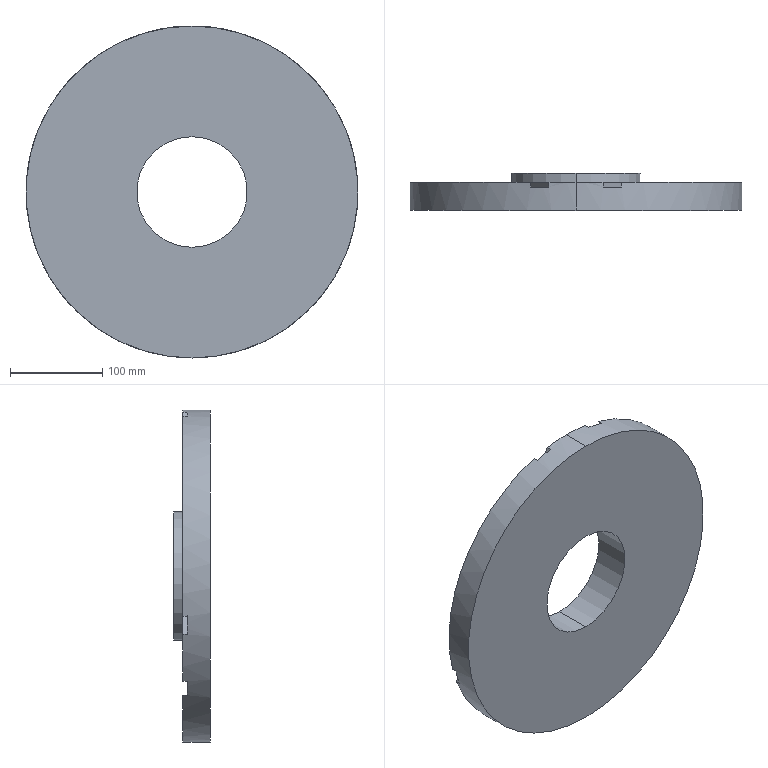Part | SolidWorks | features ICE 2, CirPattern 1, Extrusion 1 | 1 solid | 21 faces | box 360 x 40 x 360 mm | volume 2695575 mm3 | plane 15 | cylinder 6 | commonest cylinder face diameters 120 x2 140 x2 360 x2
STEP:
#1=CARTESIAN_POINT('',(0.,40.,70.));
#2=VERTEX_POINT('',#1);
#3=CARTESIAN_POINT('',(0.,40.,-70.));
#4=VERTEX_POINT('',#3);
#5=CARTESIAN_POINT('',(0.,40.,0.));
#6=DIRECTION('',(0.,1.,0.));
#7=DIRECTION('',(0.,0.,1.));
#8=AXIS2_PLACEMENT_3D('',#5,#6,#7);
#9=CIRCLE('',#8,70.);
#10=EDGE_CURVE('',#2,#4,#9,.T.);
#11=ORIENTED_EDGE('',*,*,#10,.F.);
#12=CARTESIAN_POINT('',(0.,30.,70.));
#13=VERTEX_POINT('',#12);
#14=CARTESIAN_POINT('',(0.,40.,70.));
#15=DIRECTION('',(0.,-1.,0.));
#16=VECTOR('',#15,1000.);
#17=LINE('',#14,#16);
#18=EDGE_CURVE('',#2,#13,#17,.T.);
#19=ORIENTED_EDGE('',*,*,#18,.T.);
#20=CARTESIAN_POINT('',(0.,30.,-70.));
#21=VERTEX_POINT('',#20);
#22=CARTESIAN_POINT('',(0.,30.,0.));
#23=DIRECTION('',(0.,1.,0.));
#24=DIRECTION('',(0.,0.,1.));
#25=AXIS2_PLACEMENT_3D('',#22,#23,#24);
#26=CIRCLE('',#25,70.);
#27=EDGE_CURVE('',#13,#21,#26,.T.);
#28=ORIENTED_EDGE('',*,*,#27,.T.);
#29=CARTESIAN_POINT('',(0.,40.,-70.));
#30=DIRECTION('',(0.,-1.,0.));
#31=VECTOR('',#30,1000.);
#32=LINE('',#29,#31);
#33=EDGE_CURVE('',#4,#21,#32,.T.);
#34=ORIENTED_EDGE('',*,*,#33,.F.);
#35=EDGE_LOOP('',(#11,#19,#28,#34));
#36=FACE_OUTER_BOUND('',#35,.T.);
#37=CARTESIAN_POINT('',(0.,40.,0.));
#38=DIRECTION('',(0.,-1.,0.));
#39=DIRECTION('',(0.,0.,-1.));
#40=AXIS2_PLACEMENT_3D('',#37,#38,#39);
#41=CYLINDRICAL_SURFACE('',#40,70.);
#42=ADVANCED_FACE('',(#36),#41,.T.);
#43=CARTESIAN_POINT('',(0.,40.,-60.));
#44=VERTEX_POINT('',#43);
#45=CARTESIAN_POINT('',(0.,40.,60.));
#46=VERTEX_POINT('',#45);
#47=CARTESIAN_POINT('',(0.,40.,0.));
#48=DIRECTION('',(0.,1.,0.));
#49=DIRECTION('',(0.,0.,1.));
#50=AXIS2_PLACEMENT_3D('',#47,#48,#49);
#51=CIRCLE('',#50,60.);
#52=EDGE_CURVE('',#44,#46,#51,.T.);
#53=ORIENTED_EDGE('',*,*,#52,.T.);
#54=CARTESIAN_POINT('',(0.,0.,60.));
#55=VERTEX_POINT('',#54);
#56=CARTESIAN_POINT('',(0.,30.,60.));
#57=DIRECTION('',(0.,-1.,0.));
#58=VECTOR('',#57,1000.);
#59=LINE('',#56,#58);
#60=EDGE_CURVE('',#46,#55,#59,.T.);
#61=ORIENTED_EDGE('',*,*,#60,.T.);
#62=CARTESIAN_POINT('',(0.,0.,-60.));
#63=VERTEX_POINT('',#62);
#64=CARTESIAN_POINT('',(0.,0.,0.));
#65=DIRECTION('',(0.,1.,0.));
#66=DIRECTION('',(0.,0.,1.));
#67=AXIS2_PLACEMENT_3D('',#64,#65,#66);
#68=CIRCLE('',#67,60.);
#69=EDGE_CURVE('',#63,#55,#68,.T.);
#70=ORIENTED_EDGE('',*,*,#69,.F.);
#71=CARTESIAN_POINT('',(0.,30.,-60.));
#72=DIRECTION('',(0.,-1.,0.));
#73=VECTOR('',#72,1000.);
#74=LINE('',#71,#73);
#75=EDGE_CURVE('',#44,#63,#74,.T.);
#76=ORIENTED_EDGE('',*,*,#75,.F.);
#77=EDGE_LOOP('',(#53,#61,#70,#76));
#78=FACE_OUTER_BOUND('',#77,.T.);
#79=CARTESIAN_POINT('',(0.,30.,0.));
#80=DIRECTION('',(0.,-1.,0.));
#81=DIRECTION('',(0.,0.,-1.));
#82=AXIS2_PLACEMENT_3D('',#79,#80,#81);
#83=CYLINDRICAL_SURFACE('',#82,60.);
#84=ADVANCED_FACE('',(#78),#83,.F.);
#85=CARTESIAN_POINT('',(0.,30.,180.));
#86=VERTEX_POINT('',#85);
#87=CARTESIAN_POINT('',(29.397,30.,177.583));
#88=VERTEX_POINT('',#87);
#89=CARTESIAN_POINT('',(0.,30.,0.));
#90=DIRECTION('',(0.,1.,0.));
#91=DIRECTION('',(0.,0.,1.));
#92=AXIS2_PLACEMENT_3D('',#89,#90,#91);
#93=CIRCLE('',#92,180.);
#94=EDGE_CURVE('',#86,#88,#93,.T.);
#95=ORIENTED_EDGE('',*,*,#94,.F.);
#96=CARTESIAN_POINT('',(0.,0.,180.));
#97=VERTEX_POINT('',#96);
#98=CARTESIAN_POINT('',(0.,30.,180.));
#99=DIRECTION('',(0.,-1.,0.));
#100=VECTOR('',#99,1000.);
#101=LINE('',#98,#100);
#102=EDGE_CURVE('',#86,#97,#101,.T.);
#103=ORIENTED_EDGE('',*,*,#102,.T.);
#104=CARTESIAN_POINT('',(0.,0.,-180.));
#105=VERTEX_POINT('',#104);
#106=CARTESIAN_POINT('',(0.,0.,0.));
#107=DIRECTION('',(0.,1.,0.));
#108=DIRECTION('',(0.,0.,1.));
#109=AXIS2_PLACEMENT_3D('',#106,#107,#108);
#110=CIRCLE('',#109,180.);
#111=EDGE_CURVE('',#97,#105,#110,.T.);
#112=ORIENTED_EDGE('',*,*,#111,.T.);
#113=CARTESIAN_POINT('',(0.,30.,-180.));
#114=VERTEX_POINT('',#113);
#115=CARTESIAN_POINT('',(0.,30.,-180.));
#116=DIRECTION('',(0.,-1.,0.));
#117=VECTOR('',#116,1000.);
#118=LINE('',#115,#117);
#119=EDGE_CURVE('',#114,#105,#118,.T.);
#120=ORIENTED_EDGE('',*,*,#119,.F.);
#121=CARTESIAN_POINT('',(125.277,30.,-129.25));
#122=VERTEX_POINT('',#121);
#123=CARTESIAN_POINT('',(0.,30.,0.));
#124=DIRECTION('',(0.,1.,0.));
#125=DIRECTION('',(0.,0.,1.));
#126=AXIS2_PLACEMENT_3D('',#123,#124,#125);
#127=CIRCLE('',#126,180.);
#128=EDGE_CURVE('',#122,#114,#127,.T.);
#129=ORIENTED_EDGE('',*,*,#128,.F.);
#130=CARTESIAN_POINT('',(125.277,25.,-129.25));
#131=VERTEX_POINT('',#130);
#132=CARTESIAN_POINT('',(125.277,30.,-129.25));
#133=DIRECTION('',(0.,-1.,0.));
#134=VECTOR('',#133,1000.);
#135=LINE('',#132,#134);
#136=EDGE_CURVE('',#122,#131,#135,.T.);
#137=ORIENTED_EDGE('',*,*,#136,.T.);
#138=CARTESIAN_POINT('',(139.093,25.,-114.25));
#139=VERTEX_POINT('',#138);
#140=CARTESIAN_POINT('',(0.,25.,0.));
#141=DIRECTION('',(0.,1.,0.));
#142=DIRECTION('',(0.,0.,1.));
#143=AXIS2_PLACEMENT_3D('',#140,#141,#142);
#144=CIRCLE('',#143,180.);
#145=EDGE_CURVE('',#139,#131,#144,.T.);
#146=ORIENTED_EDGE('',*,*,#145,.F.);
#147=CARTESIAN_POINT('',(139.093,30.,-114.25));
#148=VERTEX_POINT('',#147);
#149=CARTESIAN_POINT('',(139.093,30.,-114.25));
#150=DIRECTION('',(0.,1.,0.));
#151=VECTOR('',#150,1000.);
#152=LINE('',#149,#151);
#153=EDGE_CURVE('',#139,#148,#152,.T.);
#154=ORIENTED_EDGE('',*,*,#153,.T.);
#155=CARTESIAN_POINT('',(168.49,30.,-63.333));
#156=VERTEX_POINT('',#155);
#157=CARTESIAN_POINT('',(0.,30.,0.));
#158=DIRECTION('',(0.,1.,0.));
#159=DIRECTION('',(0.,0.,1.));
#160=AXIS2_PLACEMENT_3D('',#157,#158,#159);
#161=CIRCLE('',#160,180.);
#162=EDGE_CURVE('',#156,#148,#161,.T.);
#163=ORIENTED_EDGE('',*,*,#162,.F.);
#164=CARTESIAN_POINT('',(168.49,25.,-63.333));
#165=VERTEX_POINT('',#164);
#166=CARTESIAN_POINT('',(168.49,30.,-63.333));
#167=DIRECTION('',(0.,-1.,0.));
#168=VECTOR('',#167,1000.);
#169=LINE('',#166,#168);
#170=EDGE_CURVE('',#156,#165,#169,.T.);
#171=ORIENTED_EDGE('',*,*,#170,.T.);
#172=CARTESIAN_POINT('',(174.573,25.,-43.868));
#173=VERTEX_POINT('',#172);
#174=CARTESIAN_POINT('',(0.,25.,0.));
#175=DIRECTION('',(0.,1.,0.));
#176=DIRECTION('',(0.,0.,1.));
#177=AXIS2_PLACEMENT_3D('',#174,#175,#176);
#178=CIRCLE('',#177,180.);
#179=EDGE_CURVE('',#173,#165,#178,.T.);
#180=ORIENTED_EDGE('',*,*,#179,.F.);
#181=CARTESIAN_POINT('',(174.573,30.,-43.868));
#182=VERTEX_POINT('',#181);
#183=CARTESIAN_POINT('',(174.573,30.,-43.868));
#184=DIRECTION('',(0.,1.,0.));
#185=VECTOR('',#184,1000.);
#186=LINE('',#183,#185);
#187=EDGE_CURVE('',#173,#182,#186,.T.);
#188=ORIENTED_EDGE('',*,*,#187,.T.);
#189=CARTESIAN_POINT('',(49.295,30.,173.118));
#190=VERTEX_POINT('',#189);
#191=CARTESIAN_POINT('',(0.,30.,0.));
#192=DIRECTION('',(0.,1.,0.));
#193=DIRECTION('',(0.,0.,1.));
#194=AXIS2_PLACEMENT_3D('',#191,#192,#193);
#195=CIRCLE('',#194,180.);
#196=EDGE_CURVE('',#190,#182,#195,.T.);
#197=ORIENTED_EDGE('',*,*,#196,.F.);
#198=CARTESIAN_POINT('',(49.295,25.,173.118));
#199=VERTEX_POINT('',#198);
#200=CARTESIAN_POINT('',(49.295,30.,173.118));
#201=DIRECTION('',(0.,-1.,0.));
#202=VECTOR('',#201,1000.);
#203=LINE('',#200,#202);
#204=EDGE_CURVE('',#190,#199,#203,.T.);
#205=ORIENTED_EDGE('',*,*,#204,.T.);
#206=CARTESIAN_POINT('',(29.397,25.,177.583));
#207=VERTEX_POINT('',#206);
#208=CARTESIAN_POINT('',(0.,25.,0.));
#209=DIRECTION('',(0.,1.,0.));
#210=DIRECTION('',(0.,0.,1.));
#211=AXIS2_PLACEMENT_3D('',#208,#209,#210);
#212=CIRCLE('',#211,180.);
#213=EDGE_CURVE('',#207,#199,#212,.T.);
#214=ORIENTED_EDGE('',*,*,#213,.F.);
#215=CARTESIAN_POINT('',(29.397,30.,177.583));
#216=DIRECTION('',(0.,1.,0.));
#217=VECTOR('',#216,1000.);
#218=LINE('',#215,#217);
#219=EDGE_CURVE('',#207,#88,#218,.T.);
#220=ORIENTED_EDGE('',*,*,#219,.T.);
#221=EDGE_LOOP('',(#95,#103,#112,#120,#129,#137,#146,#154,#163,#171,#180,#188,#197,#205,#214,#220));
#222=FACE_OUTER_BOUND('',#221,.T.);
#223=CARTESIAN_POINT('',(0.,30.,0.));
#224=DIRECTION('',(0.,-1.,0.));
#225=DIRECTION('',(0.,0.,-1.));
#226=AXIS2_PLACEMENT_3D('',#223,#224,#225);
#227=CYLINDRICAL_SURFACE('',#226,180.);
#228=ADVANCED_FACE('',(#222),#227,.T.);
#229=CARTESIAN_POINT('',(11.596,30.,238.415));
#230=DIRECTION('',(0.5,0.,-0.866));
#231=VECTOR('',#230,1000.);
#232=LINE('',#229,#231);
#233=EDGE_CURVE('',#190,#182,#232,.T.);
#234=ORIENTED_EDGE('',*,*,#233,.F.);
#235=ORIENTED_EDGE('',*,*,#196,.T.);
#236=EDGE_LOOP('',(#234,#235));
#237=FACE_OUTER_BOUND('',#236,.T.);
#238=CARTESIAN_POINT('',(0.,30.,0.));
#239=DIRECTION('',(0.,1.,0.));
#240=DIRECTION('',(0.,0.,1.));
#241=AXIS2_PLACEMENT_3D('',#238,#239,#240);
#242=PLANE('',#241);
#243=ADVANCED_FACE('',(#237),#242,.T.);
#244=CARTESIAN_POINT('',(-174.573,30.,-43.868));
#245=VERTEX_POINT('',#244);
#246=CARTESIAN_POINT('',(-49.295,30.,173.118));
#247=VERTEX_POINT('',#246);
#248=CARTESIAN_POINT('',(-212.271,30.,-109.165));
#249=DIRECTION('',(0.5,0.,0.866));
#250=VECTOR('',#249,1000.);
#251=LINE('',#248,#250);
#252=EDGE_CURVE('',#245,#247,#251,.T.);
#253=ORIENTED_EDGE('',*,*,#252,.F.);
#254=CARTESIAN_POINT('',(0.,30.,0.));
#255=DIRECTION('',(0.,1.,0.));
#256=DIRECTION('',(0.,0.,1.));
#257=AXIS2_PLACEMENT_3D('',#254,#255,#256);
#258=CIRCLE('',#257,180.);
#259=EDGE_CURVE('',#245,#247,#258,.T.);
#260=ORIENTED_EDGE('',*,*,#259,.T.);
#261=EDGE_LOOP('',(#253,#260));
#262=FACE_OUTER_BOUND('',#261,.T.);
#263=CARTESIAN_POINT('',(0.,30.,0.));
#264=DIRECTION('',(0.,1.,0.));
#265=DIRECTION('',(0.,0.,1.));
#266=AXIS2_PLACEMENT_3D('',#263,#264,#265);
#267=PLANE('',#266);
#268=ADVANCED_FACE('',(#262),#267,.T.);
#269=CARTESIAN_POINT('',(-125.277,30.,-129.25));
#270=VERTEX_POINT('',#269);
#271=CARTESIAN_POINT('',(200.675,30.,-129.25));
#272=DIRECTION('',(-1.,0.,0.));
#273=VECTOR('',#272,1000.);
#274=LINE('',#271,#273);
#275=EDGE_CURVE('',#122,#270,#274,.T.);
#276=ORIENTED_EDGE('',*,*,#275,.F.);
#277=ORIENTED_EDGE('',*,*,#128,.T.);
#278=CARTESIAN_POINT('',(0.,30.,0.));
#279=DIRECTION('',(0.,1.,0.));
#280=DIRECTION('',(0.,0.,1.));
#281=AXIS2_PLACEMENT_3D('',#278,#279,#280);
#282=CIRCLE('',#281,180.);
#283=EDGE_CURVE('',#114,#270,#282,.T.);
#284=ORIENTED_EDGE('',*,*,#283,.T.);
#285=EDGE_LOOP('',(#276,#277,#284));
#286=FACE_OUTER_BOUND('',#285,.T.);
#287=CARTESIAN_POINT('',(0.,30.,0.));
#288=DIRECTION('',(0.,1.,0.));
#289=DIRECTION('',(0.,0.,1.));
#290=AXIS2_PLACEMENT_3D('',#287,#288,#289);
#291=PLANE('',#290);
#292=ADVANCED_FACE('',(#286),#291,.T.);
#293=CARTESIAN_POINT('',(192.249,30.,-104.485));
#294=DIRECTION('',(-0.5,0.,0.866));
#295=VECTOR('',#294,1000.);
#296=LINE('',#293,#295);
#297=EDGE_CURVE('',#156,#88,#296,.T.);
#298=ORIENTED_EDGE('',*,*,#297,.F.);
#299=ORIENTED_EDGE('',*,*,#162,.T.);
#300=CARTESIAN_POINT('',(-139.093,30.,-114.25));
#301=VERTEX_POINT('',#300);
#302=CARTESIAN_POINT('',(-186.612,30.,-114.25));
#303=DIRECTION('',(1.,0.,0.));
#304=VECTOR('',#303,1000.);
#305=LINE('',#302,#304);
#306=EDGE_CURVE('',#301,#148,#305,.T.);
#307=ORIENTED_EDGE('',*,*,#306,.F.);
#308=CARTESIAN_POINT('',(-168.49,30.,-63.333));
#309=VERTEX_POINT('',#308);
#310=CARTESIAN_POINT('',(0.,30.,0.));
#311=DIRECTION('',(0.,1.,0.));
#312=DIRECTION('',(0.,0.,1.));
#313=AXIS2_PLACEMENT_3D('',#310,#311,#312);
#314=CIRCLE('',#313,180.);
#315=EDGE_CURVE('',#301,#309,#314,.T.);
#316=ORIENTED_EDGE('',*,*,#315,.T.);
#317=CARTESIAN_POINT('',(-29.397,30.,177.583));
#318=VERTEX_POINT('',#317);
#319=CARTESIAN_POINT('',(-5.638,30.,218.735));
#320=DIRECTION('',(-0.5,0.,-0.866));
#321=VECTOR('',#320,1000.);
#322=LINE('',#319,#321);
#323=EDGE_CURVE('',#318,#309,#322,.T.);
#324=ORIENTED_EDGE('',*,*,#323,.F.);
#325=CARTESIAN_POINT('',(0.,30.,0.));
#326=DIRECTION('',(0.,1.,0.));
#327=DIRECTION('',(0.,0.,1.));
#328=AXIS2_PLACEMENT_3D('',#325,#326,#327);
#329=CIRCLE('',#328,180.);
#330=EDGE_CURVE('',#318,#86,#329,.T.);
#331=ORIENTED_EDGE('',*,*,#330,.T.);
#332=ORIENTED_EDGE('',*,*,#94,.T.);
#333=EDGE_LOOP('',(#298,#299,#307,#316,#324,#331,#332));
#334=FACE_OUTER_BOUND('',#333,.T.);
#335=CARTESIAN_POINT('',(0.,30.,0.));
#336=DIRECTION('',(0.,1.,0.));
#337=DIRECTION('',(0.,0.,1.));
#338=AXIS2_PLACEMENT_3D('',#335,#336,#337);
#339=CIRCLE('',#338,70.);
#340=EDGE_CURVE('',#21,#13,#339,.T.);
#341=ORIENTED_EDGE('',*,*,#340,.F.);
#342=ORIENTED_EDGE('',*,*,#27,.F.);
#343=EDGE_LOOP('',(#341,#342));
#344=FACE_BOUND('',#343,.T.);
#345=CARTESIAN_POINT('',(0.,30.,0.));
#346=DIRECTION('',(0.,1.,0.));
#347=DIRECTION('',(0.,0.,1.));
#348=AXIS2_PLACEMENT_3D('',#345,#346,#347);
#349=PLANE('',#348);
#350=ADVANCED_FACE('',(#334,#344),#349,.T.);
#351=CARTESIAN_POINT('',(0.,0.,0.));
#352=DIRECTION('',(0.,1.,0.));
#353=DIRECTION('',(0.,0.,1.));
#354=AXIS2_PLACEMENT_3D('',#351,#352,#353);
#355=CIRCLE('',#354,180.);
#356=EDGE_CURVE('',#105,#97,#355,.T.);
#357=ORIENTED_EDGE('',*,*,#356,.F.);
#358=ORIENTED_EDGE('',*,*,#111,.F.);
#359=EDGE_LOOP('',(#357,#358));
#360=FACE_OUTER_BOUND('',#359,.T.);
#361=ORIENTED_EDGE('',*,*,#69,.T.);
#362=CARTESIAN_POINT('',(0.,0.,0.));
#363=DIRECTION('',(0.,1.,0.));
#364=DIRECTION('',(0.,0.,1.));
#365=AXIS2_PLACEMENT_3D('',#362,#363,#364);
#366=CIRCLE('',#365,60.);
#367=EDGE_CURVE('',#55,#63,#366,.T.);
#368=ORIENTED_EDGE('',*,*,#367,.T.);
#369=EDGE_LOOP('',(#361,#368));
#370=FACE_BOUND('',#369,.T.);
#371=CARTESIAN_POINT('',(0.,0.,0.));
#372=DIRECTION('',(0.,1.,0.));
#373=DIRECTION('',(0.,0.,1.));
#374=AXIS2_PLACEMENT_3D('',#371,#372,#373);
#375=PLANE('',#374);
#376=ADVANCED_FACE('',(#360,#370),#375,.F.);
#377=ORIENTED_EDGE('',*,*,#102,.F.);
#378=ORIENTED_EDGE('',*,*,#330,.F.);
#379=CARTESIAN_POINT('',(-29.397,25.,177.583));
#380=VERTEX_POINT('',#379);
#381=CARTESIAN_POINT('',(-29.397,30.,177.583));
#382=DIRECTION('',(0.,-1.,0.));
#383=VECTOR('',#382,1000.);
#384=LINE('',#381,#383);
#385=EDGE_CURVE('',#318,#380,#384,.T.);
#386=ORIENTED_EDGE('',*,*,#385,.T.);
#387=CARTESIAN_POINT('',(-49.295,25.,173.118));
#388=VERTEX_POINT('',#387);
#389=CARTESIAN_POINT('',(0.,25.,0.));
#390=DIRECTION('',(0.,1.,0.));
#391=DIRECTION('',(0.,0.,1.));
#392=AXIS2_PLACEMENT_3D('',#389,#390,#391);
#393=CIRCLE('',#392,180.);
#394=EDGE_CURVE('',#388,#380,#393,.T.);
#395=ORIENTED_EDGE('',*,*,#394,.F.);
#396=CARTESIAN_POINT('',(-49.295,30.,173.118));
#397=DIRECTION('',(0.,1.,0.));
#398=VECTOR('',#397,1000.);
#399=LINE('',#396,#398);
#400=EDGE_CURVE('',#388,#247,#399,.T.);
#401=ORIENTED_EDGE('',*,*,#400,.T.);
#402=ORIENTED_EDGE('',*,*,#259,.F.);
#403=CARTESIAN_POINT('',(-174.573,25.,-43.868));
#404=VERTEX_POINT('',#403);
#405=CARTESIAN_POINT('',(-174.573,30.,-43.868));
#406=DIRECTION('',(0.,-1.,0.));
#407=VECTOR('',#406,1000.);
#408=LINE('',#405,#407);
#409=EDGE_CURVE('',#245,#404,#408,.T.);
#410=ORIENTED_EDGE('',*,*,#409,.T.);
#411=CARTESIAN_POINT('',(-168.49,25.,-63.333));
#412=VERTEX_POINT('',#411);
#413=CARTESIAN_POINT('',(0.,25.,0.));
#414=DIRECTION('',(0.,1.,0.));
#415=DIRECTION('',(0.,0.,1.));
#416=AXIS2_PLACEMENT_3D('',#413,#414,#415);
#417=CIRCLE('',#416,180.);
#418=EDGE_CURVE('',#412,#404,#417,.T.);
#419=ORIENTED_EDGE('',*,*,#418,.F.);
#420=CARTESIAN_POINT('',(-168.49,30.,-63.333));
#421=DIRECTION('',(0.,1.,0.));
#422=VECTOR('',#421,1000.);
#423=LINE('',#420,#422);
#424=EDGE_CURVE('',#412,#309,#423,.T.);
#425=ORIENTED_EDGE('',*,*,#424,.T.);
#426=ORIENTED_EDGE('',*,*,#315,.F.);
#427=CARTESIAN_POINT('',(-139.093,25.,-114.25));
#428=VERTEX_POINT('',#427);
#429=CARTESIAN_POINT('',(-139.093,30.,-114.25));
#430=DIRECTION('',(0.,-1.,0.));
#431=VECTOR('',#430,1000.);
#432=LINE('',#429,#431);
#433=EDGE_CURVE('',#301,#428,#432,.T.);
#434=ORIENTED_EDGE('',*,*,#433,.T.);
#435=CARTESIAN_POINT('',(-125.277,25.,-129.25));
#436=VERTEX_POINT('',#435);
#437=CARTESIAN_POINT('',(0.,25.,0.));
#438=DIRECTION('',(0.,1.,0.));
#439=DIRECTION('',(0.,0.,1.));
#440=AXIS2_PLACEMENT_3D('',#437,#438,#439);
#441=CIRCLE('',#440,180.);
#442=EDGE_CURVE('',#436,#428,#441,.T.);
#443=ORIENTED_EDGE('',*,*,#442,.F.);
#444=CARTESIAN_POINT('',(-125.277,30.,-129.25));
#445=DIRECTION('',(0.,1.,0.));
#446=VECTOR('',#445,1000.);
#447=LINE('',#444,#446);
#448=EDGE_CURVE('',#436,#270,#447,.T.);
#449=ORIENTED_EDGE('',*,*,#448,.T.);
#450=ORIENTED_EDGE('',*,*,#283,.F.);
#451=ORIENTED_EDGE('',*,*,#119,.T.);
#452=ORIENTED_EDGE('',*,*,#356,.T.);
#453=EDGE_LOOP('',(#377,#378,#386,#395,#401,#402,#410,#419,#425,#426,#434,#443,#449,#450,#451,#452));
#454=FACE_OUTER_BOUND('',#453,.T.);
#455=CARTESIAN_POINT('',(0.,30.,0.));
#456=DIRECTION('',(0.,-1.,0.));
#457=DIRECTION('',(0.,0.,-1.));
#458=AXIS2_PLACEMENT_3D('',#455,#456,#457);
#459=CYLINDRICAL_SURFACE('',#458,180.);
#460=ADVANCED_FACE('',(#454),#459,.T.);
#461=ORIENTED_EDGE('',*,*,#60,.F.);
#462=CARTESIAN_POINT('',(0.,40.,0.));
#463=DIRECTION('',(0.,1.,0.));
#464=DIRECTION('',(0.,0.,1.));
#465=AXIS2_PLACEMENT_3D('',#462,#463,#464);
#466=CIRCLE('',#465,60.);
#467=EDGE_CURVE('',#46,#44,#466,.T.);
#468=ORIENTED_EDGE('',*,*,#467,.T.);
#469=ORIENTED_EDGE('',*,*,#75,.T.);
#470=ORIENTED_EDGE('',*,*,#367,.F.);
#471=EDGE_LOOP('',(#461,#468,#469,#470));
#472=FACE_OUTER_BOUND('',#471,.T.);
#473=CARTESIAN_POINT('',(0.,30.,0.));
#474=DIRECTION('',(0.,-1.,0.));
#475=DIRECTION('',(0.,0.,-1.));
#476=AXIS2_PLACEMENT_3D('',#473,#474,#475);
#477=CYLINDRICAL_SURFACE('',#476,60.);
#478=ADVANCED_FACE('',(#472),#477,.F.);
#479=CARTESIAN_POINT('',(0.,40.,0.));
#480=DIRECTION('',(0.,1.,0.));
#481=DIRECTION('',(0.,0.,1.));
#482=AXIS2_PLACEMENT_3D('',#479,#480,#481);
#483=CIRCLE('',#482,70.);
#484=EDGE_CURVE('',#4,#2,#483,.T.);
#485=ORIENTED_EDGE('',*,*,#484,.T.);
#486=ORIENTED_EDGE('',*,*,#10,.T.);
#487=EDGE_LOOP('',(#485,#486));
#488=FACE_OUTER_BOUND('',#487,.T.);
#489=ORIENTED_EDGE('',*,*,#52,.F.);
#490=ORIENTED_EDGE('',*,*,#467,.F.);
#491=EDGE_LOOP('',(#489,#490));
#492=FACE_BOUND('',#491,.T.);
#493=CARTESIAN_POINT('',(0.,40.,0.));
#494=DIRECTION('',(0.,1.,0.));
#495=DIRECTION('',(0.,0.,1.));
#496=AXIS2_PLACEMENT_3D('',#493,#494,#495);
#497=PLANE('',#496);
#498=ADVANCED_FACE('',(#488,#492),#497,.T.);
#499=ORIENTED_EDGE('',*,*,#18,.F.);
#500=ORIENTED_EDGE('',*,*,#484,.F.);
#501=ORIENTED_EDGE('',*,*,#33,.T.);
#502=ORIENTED_EDGE('',*,*,#340,.T.);
#503=EDGE_LOOP('',(#499,#500,#501,#502));
#504=FACE_OUTER_BOUND('',#503,.T.);
#505=CARTESIAN_POINT('',(0.,40.,0.));
#506=DIRECTION('',(0.,-1.,0.));
#507=DIRECTION('',(0.,0.,-1.));
#508=AXIS2_PLACEMENT_3D('',#505,#506,#507);
#509=CYLINDRICAL_SURFACE('',#508,70.);
#510=ADVANCED_FACE('',(#504),#509,.T.);
#511=ORIENTED_EDGE('',*,*,#275,.T.);
#512=ORIENTED_EDGE('',*,*,#448,.F.);
#513=CARTESIAN_POINT('',(200.675,25.,-129.25));
#514=DIRECTION('',(-1.,0.,0.));
#515=VECTOR('',#514,1000.);
#516=LINE('',#513,#515);
#517=EDGE_CURVE('',#131,#436,#516,.T.);
#518=ORIENTED_EDGE('',*,*,#517,.F.);
#519=ORIENTED_EDGE('',*,*,#136,.F.);
#520=EDGE_LOOP('',(#511,#512,#518,#519));
#521=FACE_OUTER_BOUND('',#520,.T.);
#522=CARTESIAN_POINT('',(200.675,25.,-129.25));
#523=DIRECTION('',(0.,0.,-1.));
#524=DIRECTION('',(-1.,0.,0.));
#525=AXIS2_PLACEMENT_3D('',#522,#523,#524);
#526=PLANE('',#525);
#527=ADVANCED_FACE('',(#521),#526,.F.);
#528=ORIENTED_EDGE('',*,*,#306,.T.);
#529=ORIENTED_EDGE('',*,*,#153,.F.);
#530=CARTESIAN_POINT('',(-186.612,25.,-114.25));
#531=DIRECTION('',(1.,0.,0.));
#532=VECTOR('',#531,1000.);
#533=LINE('',#530,#532);
#534=EDGE_CURVE('',#428,#139,#533,.T.);
#535=ORIENTED_EDGE('',*,*,#534,.F.);
#536=ORIENTED_EDGE('',*,*,#433,.F.);
#537=EDGE_LOOP('',(#528,#529,#535,#536));
#538=FACE_OUTER_BOUND('',#537,.T.);
#539=CARTESIAN_POINT('',(-186.612,25.,-114.25));
#540=DIRECTION('',(0.,0.,1.));
#541=DIRECTION('',(1.,0.,0.));
#542=AXIS2_PLACEMENT_3D('',#539,#540,#541);
#543=PLANE('',#542);
#544=ADVANCED_FACE('',(#538),#543,.F.);
#545=ORIENTED_EDGE('',*,*,#145,.T.);
#546=ORIENTED_EDGE('',*,*,#517,.T.);
#547=ORIENTED_EDGE('',*,*,#442,.T.);
#548=ORIENTED_EDGE('',*,*,#534,.T.);
#549=EDGE_LOOP('',(#545,#546,#547,#548));
#550=FACE_OUTER_BOUND('',#549,.T.);
#551=CARTESIAN_POINT('',(0.,25.,0.));
#552=DIRECTION('',(0.,1.,0.));
#553=DIRECTION('',(0.,0.,1.));
#554=AXIS2_PLACEMENT_3D('',#551,#552,#553);
#555=PLANE('',#554);
#556=ADVANCED_FACE('',(#550),#555,.T.);
#557=ORIENTED_EDGE('',*,*,#252,.T.);
#558=ORIENTED_EDGE('',*,*,#400,.F.);
#559=CARTESIAN_POINT('',(-212.271,25.,-109.165));
#560=DIRECTION('',(0.5,0.,0.866));
#561=VECTOR('',#560,1000.);
#562=LINE('',#559,#561);
#563=EDGE_CURVE('',#404,#388,#562,.T.);
#564=ORIENTED_EDGE('',*,*,#563,.F.);
#565=ORIENTED_EDGE('',*,*,#409,.F.);
#566=EDGE_LOOP('',(#557,#558,#564,#565));
#567=FACE_OUTER_BOUND('',#566,.T.);
#568=CARTESIAN_POINT('',(-212.271,25.,-109.165));
#569=DIRECTION('',(-0.866,0.,0.5));
#570=DIRECTION('',(0.5,0.,0.866));
#571=AXIS2_PLACEMENT_3D('',#568,#569,#570);
#572=PLANE('',#571);
#573=ADVANCED_FACE('',(#567),#572,.F.);
#574=ORIENTED_EDGE('',*,*,#323,.T.);
#575=ORIENTED_EDGE('',*,*,#424,.F.);
#576=CARTESIAN_POINT('',(-5.638,25.,218.735));
#577=DIRECTION('',(-0.5,0.,-0.866));
#578=VECTOR('',#577,1000.);
#579=LINE('',#576,#578);
#580=EDGE_CURVE('',#380,#412,#579,.T.);
#581=ORIENTED_EDGE('',*,*,#580,.F.);
#582=ORIENTED_EDGE('',*,*,#385,.F.);
#583=EDGE_LOOP('',(#574,#575,#581,#582));
#584=FACE_OUTER_BOUND('',#583,.T.);
#585=CARTESIAN_POINT('',(-5.638,25.,218.735));
#586=DIRECTION('',(0.866,0.,-0.5));
#587=DIRECTION('',(-0.5,0.,-0.866));
#588=AXIS2_PLACEMENT_3D('',#585,#586,#587);
#589=PLANE('',#588);
#590=ADVANCED_FACE('',(#584),#589,.F.);
#591=ORIENTED_EDGE('',*,*,#418,.T.);
#592=ORIENTED_EDGE('',*,*,#563,.T.);
#593=ORIENTED_EDGE('',*,*,#394,.T.);
#594=ORIENTED_EDGE('',*,*,#580,.T.);
#595=EDGE_LOOP('',(#591,#592,#593,#594));
#596=FACE_OUTER_BOUND('',#595,.T.);
#597=CARTESIAN_POINT('',(0.,25.,0.));
#598=DIRECTION('',(0.,1.,0.));
#599=DIRECTION('',(0.866,0.,-0.5));
#600=AXIS2_PLACEMENT_3D('',#597,#598,#599);
#601=PLANE('',#600);
#602=ADVANCED_FACE('',(#596),#601,.T.);
#603=ORIENTED_EDGE('',*,*,#233,.T.);
#604=ORIENTED_EDGE('',*,*,#187,.F.);
#605=CARTESIAN_POINT('',(11.596,25.,238.415));
#606=DIRECTION('',(0.5,0.,-0.866));
#607=VECTOR('',#606,1000.);
#608=LINE('',#605,#607);
#609=EDGE_CURVE('',#199,#173,#608,.T.);
#610=ORIENTED_EDGE('',*,*,#609,.F.);
#611=ORIENTED_EDGE('',*,*,#204,.F.);
#612=EDGE_LOOP('',(#603,#604,#610,#611));
#613=FACE_OUTER_BOUND('',#612,.T.);
#614=CARTESIAN_POINT('',(11.596,25.,238.415));
#615=DIRECTION('',(0.866,0.,0.5));
#616=DIRECTION('',(0.5,0.,-0.866));
#617=AXIS2_PLACEMENT_3D('',#614,#615,#616);
#618=PLANE('',#617);
#619=ADVANCED_FACE('',(#613),#618,.F.);
#620=ORIENTED_EDGE('',*,*,#297,.T.);
#621=ORIENTED_EDGE('',*,*,#219,.F.);
#622=CARTESIAN_POINT('',(192.249,25.,-104.485));
#623=DIRECTION('',(-0.5,0.,0.866));
#624=VECTOR('',#623,1000.);
#625=LINE('',#622,#624);
#626=EDGE_CURVE('',#165,#207,#625,.T.);
#627=ORIENTED_EDGE('',*,*,#626,.F.);
#628=ORIENTED_EDGE('',*,*,#170,.F.);
#629=EDGE_LOOP('',(#620,#621,#627,#628));
#630=FACE_OUTER_BOUND('',#629,.T.);
#631=CARTESIAN_POINT('',(192.249,25.,-104.485));
#632=DIRECTION('',(-0.866,0.,-0.5));
#633=DIRECTION('',(-0.5,0.,0.866));
#634=AXIS2_PLACEMENT_3D('',#631,#632,#633);
#635=PLANE('',#634);
#636=ADVANCED_FACE('',(#630),#635,.F.);
#637=ORIENTED_EDGE('',*,*,#213,.T.);
#638=ORIENTED_EDGE('',*,*,#609,.T.);
#639=ORIENTED_EDGE('',*,*,#179,.T.);
#640=ORIENTED_EDGE('',*,*,#626,.T.);
#641=EDGE_LOOP('',(#637,#638,#639,#640));
#642=FACE_OUTER_BOUND('',#641,.T.);
#643=CARTESIAN_POINT('',(0.,25.,0.));
#644=DIRECTION('',(0.,1.,0.));
#645=DIRECTION('',(-0.866,0.,-0.5));
#646=AXIS2_PLACEMENT_3D('',#643,#644,#645);
#647=PLANE('',#646);
#648=ADVANCED_FACE('',(#642),#647,.T.);
#649=CLOSED_SHELL('',(#42,#84,#228,#243,#268,#292,#350,#376,#460,#478,#498,#510,#527,#544,#556,#573,#590,#602,#619,#636,#648));
#650=MANIFOLD_SOLID_BREP('',#649);
#651=CARTESIAN_POINT('',(0.,0.,0.));
#652=DIRECTION('',(0.,0.,1.));
#653=DIRECTION('',(1.,0.,0.));
#654=AXIS2_PLACEMENT_3D('',#651,#652,#653);
#655=(LENGTH_UNIT()NAMED_UNIT(*)SI_UNIT(.MILLI.,.METRE.));
#656=UNCERTAINTY_MEASURE_WITH_UNIT(LENGTH_MEASURE(0.00001),#655,'','');
#657=(NAMED_UNIT(*)PLANE_ANGLE_UNIT()SI_UNIT($,.RADIAN.));
#658=(NAMED_UNIT(*)SI_UNIT($,.STERADIAN.)SOLID_ANGLE_UNIT());
#659=(GEOMETRIC_REPRESENTATION_CONTEXT(3)GLOBAL_UNCERTAINTY_ASSIGNED_CONTEXT((#656))GLOBAL_UNIT_ASSIGNED_CONTEXT((#655,#657,#658))REPRESENTATION_CONTEXT('',''));
#660=ADVANCED_BREP_SHAPE_REPRESENTATION('',(#650,#654),#659);